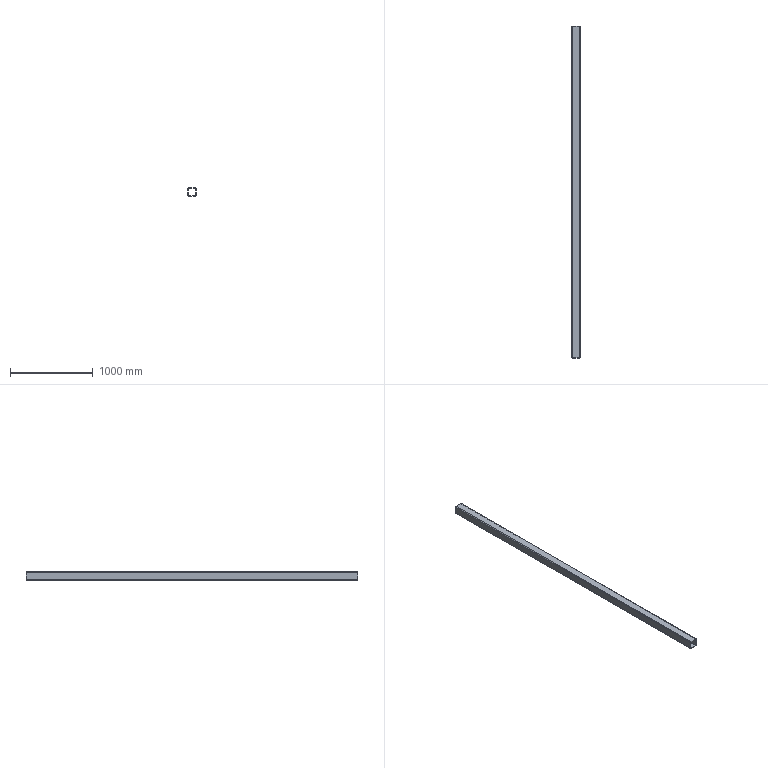Part | SolidWorks | features Extrusion 1 | 1 solid | 18 faces | box 100 x 4000 x 100 mm | volume 9368302 mm3 | plane 10 | cylinder 8 | commonest cylinder face diameters 12.6 x4 15.75 x4
STEP:
#1=CARTESIAN_POINT('',(100.,2000.,-90.6));
#2=VERTEX_POINT('',#1);
#3=CARTESIAN_POINT('',(92.125,2000.,-98.475));
#4=VERTEX_POINT('',#3);
#5=CARTESIAN_POINT('',(92.125,2000.,-90.6));
#6=DIRECTION('',(0.,1.,0.));
#7=DIRECTION('',(0.,0.,1.));
#8=AXIS2_PLACEMENT_3D('',#5,#6,#7);
#9=CIRCLE('',#8,7.875);
#10=EDGE_CURVE('',#2,#4,#9,.T.);
#11=ORIENTED_EDGE('',*,*,#10,.T.);
#12=CARTESIAN_POINT('',(7.875,2000.,-98.475));
#13=VERTEX_POINT('',#12);
#14=CARTESIAN_POINT('',(92.125,2000.,-98.475));
#15=DIRECTION('',(-1.,0.,0.));
#16=VECTOR('',#15,1000.);
#17=LINE('',#14,#16);
#18=EDGE_CURVE('',#4,#13,#17,.T.);
#19=ORIENTED_EDGE('',*,*,#18,.T.);
#20=CARTESIAN_POINT('',(0.,2000.,-90.6));
#21=VERTEX_POINT('',#20);
#22=CARTESIAN_POINT('',(7.875,2000.,-90.6));
#23=DIRECTION('',(0.,1.,0.));
#24=DIRECTION('',(0.,0.,1.));
#25=AXIS2_PLACEMENT_3D('',#22,#23,#24);
#26=CIRCLE('',#25,7.875);
#27=EDGE_CURVE('',#13,#21,#26,.T.);
#28=ORIENTED_EDGE('',*,*,#27,.T.);
#29=CARTESIAN_POINT('',(0.,2000.,-6.35));
#30=VERTEX_POINT('',#29);
#31=CARTESIAN_POINT('',(0.,2000.,-6.35));
#32=DIRECTION('',(0.,0.,1.));
#33=VECTOR('',#32,1000.);
#34=LINE('',#31,#33);
#35=EDGE_CURVE('',#21,#30,#34,.T.);
#36=ORIENTED_EDGE('',*,*,#35,.T.);
#37=CARTESIAN_POINT('',(7.875,2000.,1.525));
#38=VERTEX_POINT('',#37);
#39=CARTESIAN_POINT('',(7.875,2000.,-6.35));
#40=DIRECTION('',(0.,1.,0.));
#41=DIRECTION('',(0.,0.,1.));
#42=AXIS2_PLACEMENT_3D('',#39,#40,#41);
#43=CIRCLE('',#42,7.875);
#44=EDGE_CURVE('',#30,#38,#43,.T.);
#45=ORIENTED_EDGE('',*,*,#44,.T.);
#46=CARTESIAN_POINT('',(92.125,2000.,1.525));
#47=VERTEX_POINT('',#46);
#48=CARTESIAN_POINT('',(7.875,2000.,1.525));
#49=DIRECTION('',(1.,0.,0.));
#50=VECTOR('',#49,1000.);
#51=LINE('',#48,#50);
#52=EDGE_CURVE('',#38,#47,#51,.T.);
#53=ORIENTED_EDGE('',*,*,#52,.T.);
#54=CARTESIAN_POINT('',(100.,2000.,-6.35));
#55=VERTEX_POINT('',#54);
#56=CARTESIAN_POINT('',(92.125,2000.,-6.35));
#57=DIRECTION('',(0.,1.,0.));
#58=DIRECTION('',(0.,0.,1.));
#59=AXIS2_PLACEMENT_3D('',#56,#57,#58);
#60=CIRCLE('',#59,7.875);
#61=EDGE_CURVE('',#47,#55,#60,.T.);
#62=ORIENTED_EDGE('',*,*,#61,.T.);
#63=CARTESIAN_POINT('',(100.,2000.,-90.6));
#64=DIRECTION('',(0.,0.,-1.));
#65=VECTOR('',#64,1000.);
#66=LINE('',#63,#65);
#67=EDGE_CURVE('',#55,#2,#66,.T.);
#68=ORIENTED_EDGE('',*,*,#67,.T.);
#69=EDGE_LOOP('',(#11,#19,#28,#36,#45,#53,#62,#68));
#70=FACE_OUTER_BOUND('',#69,.T.);
#71=CARTESIAN_POINT('',(6.3,2000.,-85.875));
#72=VERTEX_POINT('',#71);
#73=CARTESIAN_POINT('',(6.3,2000.,-11.075));
#74=VERTEX_POINT('',#73);
#75=CARTESIAN_POINT('',(6.3,2000.,-11.075));
#76=DIRECTION('',(0.,0.,1.));
#77=VECTOR('',#76,1000.);
#78=LINE('',#75,#77);
#79=EDGE_CURVE('',#72,#74,#78,.T.);
#80=ORIENTED_EDGE('',*,*,#79,.F.);
#81=CARTESIAN_POINT('',(12.6,2000.,-92.175));
#82=VERTEX_POINT('',#81);
#83=CARTESIAN_POINT('',(12.6,2000.,-85.875));
#84=DIRECTION('',(0.,1.,0.));
#85=DIRECTION('',(0.,0.,1.));
#86=AXIS2_PLACEMENT_3D('',#83,#84,#85);
#87=CIRCLE('',#86,6.3);
#88=EDGE_CURVE('',#82,#72,#87,.T.);
#89=ORIENTED_EDGE('',*,*,#88,.F.);
#90=CARTESIAN_POINT('',(87.4,2000.,-92.175));
#91=VERTEX_POINT('',#90);
#92=CARTESIAN_POINT('',(87.4,2000.,-92.175));
#93=DIRECTION('',(-1.,0.,0.));
#94=VECTOR('',#93,1000.);
#95=LINE('',#92,#94);
#96=EDGE_CURVE('',#91,#82,#95,.T.);
#97=ORIENTED_EDGE('',*,*,#96,.F.);
#98=CARTESIAN_POINT('',(93.7,2000.,-85.875));
#99=VERTEX_POINT('',#98);
#100=CARTESIAN_POINT('',(87.4,2000.,-85.875));
#101=DIRECTION('',(0.,1.,0.));
#102=DIRECTION('',(0.,0.,1.));
#103=AXIS2_PLACEMENT_3D('',#100,#101,#102);
#104=CIRCLE('',#103,6.3);
#105=EDGE_CURVE('',#99,#91,#104,.T.);
#106=ORIENTED_EDGE('',*,*,#105,.F.);
#107=CARTESIAN_POINT('',(93.7,2000.,-11.075));
#108=VERTEX_POINT('',#107);
#109=CARTESIAN_POINT('',(93.7,2000.,-85.875));
#110=DIRECTION('',(0.,0.,-1.));
#111=VECTOR('',#110,1000.);
#112=LINE('',#109,#111);
#113=EDGE_CURVE('',#108,#99,#112,.T.);
#114=ORIENTED_EDGE('',*,*,#113,.F.);
#115=CARTESIAN_POINT('',(87.4,2000.,-4.775));
#116=VERTEX_POINT('',#115);
#117=CARTESIAN_POINT('',(87.4,2000.,-11.075));
#118=DIRECTION('',(0.,1.,0.));
#119=DIRECTION('',(0.,0.,1.));
#120=AXIS2_PLACEMENT_3D('',#117,#118,#119);
#121=CIRCLE('',#120,6.3);
#122=EDGE_CURVE('',#116,#108,#121,.T.);
#123=ORIENTED_EDGE('',*,*,#122,.F.);
#124=CARTESIAN_POINT('',(12.6,2000.,-4.775));
#125=VERTEX_POINT('',#124);
#126=CARTESIAN_POINT('',(12.6,2000.,-4.775));
#127=DIRECTION('',(1.,0.,0.));
#128=VECTOR('',#127,1000.);
#129=LINE('',#126,#128);
#130=EDGE_CURVE('',#125,#116,#129,.T.);
#131=ORIENTED_EDGE('',*,*,#130,.F.);
#132=CARTESIAN_POINT('',(12.6,2000.,-11.075));
#133=DIRECTION('',(0.,1.,0.));
#134=DIRECTION('',(0.,0.,1.));
#135=AXIS2_PLACEMENT_3D('',#132,#133,#134);
#136=CIRCLE('',#135,6.3);
#137=EDGE_CURVE('',#74,#125,#136,.T.);
#138=ORIENTED_EDGE('',*,*,#137,.F.);
#139=EDGE_LOOP('',(#80,#89,#97,#106,#114,#123,#131,#138));
#140=FACE_BOUND('',#139,.T.);
#141=CARTESIAN_POINT('',(92.125,2000.,-90.6));
#142=DIRECTION('',(0.,1.,0.));
#143=DIRECTION('',(0.,0.,1.));
#144=AXIS2_PLACEMENT_3D('',#141,#142,#143);
#145=PLANE('',#144);
#146=ADVANCED_FACE('',(#70,#140),#145,.T.);
#147=CARTESIAN_POINT('',(100.,-2000.,-90.6));
#148=VERTEX_POINT('',#147);
#149=CARTESIAN_POINT('',(92.125,-2000.,-98.475));
#150=VERTEX_POINT('',#149);
#151=CARTESIAN_POINT('',(92.125,-2000.,-90.6));
#152=DIRECTION('',(0.,1.,0.));
#153=DIRECTION('',(0.,0.,1.));
#154=AXIS2_PLACEMENT_3D('',#151,#152,#153);
#155=CIRCLE('',#154,7.875);
#156=EDGE_CURVE('',#148,#150,#155,.T.);
#157=ORIENTED_EDGE('',*,*,#156,.F.);
#158=CARTESIAN_POINT('',(100.,-2000.,-6.35));
#159=VERTEX_POINT('',#158);
#160=CARTESIAN_POINT('',(100.,-2000.,-90.6));
#161=DIRECTION('',(0.,0.,-1.));
#162=VECTOR('',#161,1000.);
#163=LINE('',#160,#162);
#164=EDGE_CURVE('',#159,#148,#163,.T.);
#165=ORIENTED_EDGE('',*,*,#164,.F.);
#166=CARTESIAN_POINT('',(92.125,-2000.,1.525));
#167=VERTEX_POINT('',#166);
#168=CARTESIAN_POINT('',(92.125,-2000.,-6.35));
#169=DIRECTION('',(0.,1.,0.));
#170=DIRECTION('',(0.,0.,1.));
#171=AXIS2_PLACEMENT_3D('',#168,#169,#170);
#172=CIRCLE('',#171,7.875);
#173=EDGE_CURVE('',#167,#159,#172,.T.);
#174=ORIENTED_EDGE('',*,*,#173,.F.);
#175=CARTESIAN_POINT('',(7.875,-2000.,1.525));
#176=VERTEX_POINT('',#175);
#177=CARTESIAN_POINT('',(7.875,-2000.,1.525));
#178=DIRECTION('',(1.,0.,0.));
#179=VECTOR('',#178,1000.);
#180=LINE('',#177,#179);
#181=EDGE_CURVE('',#176,#167,#180,.T.);
#182=ORIENTED_EDGE('',*,*,#181,.F.);
#183=CARTESIAN_POINT('',(0.,-2000.,-6.35));
#184=VERTEX_POINT('',#183);
#185=CARTESIAN_POINT('',(7.875,-2000.,-6.35));
#186=DIRECTION('',(0.,1.,0.));
#187=DIRECTION('',(0.,0.,1.));
#188=AXIS2_PLACEMENT_3D('',#185,#186,#187);
#189=CIRCLE('',#188,7.875);
#190=EDGE_CURVE('',#184,#176,#189,.T.);
#191=ORIENTED_EDGE('',*,*,#190,.F.);
#192=CARTESIAN_POINT('',(0.,-2000.,-90.6));
#193=VERTEX_POINT('',#192);
#194=CARTESIAN_POINT('',(0.,-2000.,-6.35));
#195=DIRECTION('',(0.,0.,1.));
#196=VECTOR('',#195,1000.);
#197=LINE('',#194,#196);
#198=EDGE_CURVE('',#193,#184,#197,.T.);
#199=ORIENTED_EDGE('',*,*,#198,.F.);
#200=CARTESIAN_POINT('',(7.875,-2000.,-98.475));
#201=VERTEX_POINT('',#200);
#202=CARTESIAN_POINT('',(7.875,-2000.,-90.6));
#203=DIRECTION('',(0.,1.,0.));
#204=DIRECTION('',(0.,0.,1.));
#205=AXIS2_PLACEMENT_3D('',#202,#203,#204);
#206=CIRCLE('',#205,7.875);
#207=EDGE_CURVE('',#201,#193,#206,.T.);
#208=ORIENTED_EDGE('',*,*,#207,.F.);
#209=CARTESIAN_POINT('',(92.125,-2000.,-98.475));
#210=DIRECTION('',(-1.,0.,0.));
#211=VECTOR('',#210,1000.);
#212=LINE('',#209,#211);
#213=EDGE_CURVE('',#150,#201,#212,.T.);
#214=ORIENTED_EDGE('',*,*,#213,.F.);
#215=EDGE_LOOP('',(#157,#165,#174,#182,#191,#199,#208,#214));
#216=FACE_OUTER_BOUND('',#215,.T.);
#217=CARTESIAN_POINT('',(12.6,-2000.,-92.175));
#218=VERTEX_POINT('',#217);
#219=CARTESIAN_POINT('',(6.3,-2000.,-85.875));
#220=VERTEX_POINT('',#219);
#221=CARTESIAN_POINT('',(12.6,-2000.,-85.875));
#222=DIRECTION('',(0.,1.,0.));
#223=DIRECTION('',(0.,0.,1.));
#224=AXIS2_PLACEMENT_3D('',#221,#222,#223);
#225=CIRCLE('',#224,6.3);
#226=EDGE_CURVE('',#218,#220,#225,.T.);
#227=ORIENTED_EDGE('',*,*,#226,.T.);
#228=CARTESIAN_POINT('',(6.3,-2000.,-11.075));
#229=VERTEX_POINT('',#228);
#230=CARTESIAN_POINT('',(6.3,-2000.,-11.075));
#231=DIRECTION('',(0.,0.,1.));
#232=VECTOR('',#231,1000.);
#233=LINE('',#230,#232);
#234=EDGE_CURVE('',#220,#229,#233,.T.);
#235=ORIENTED_EDGE('',*,*,#234,.T.);
#236=CARTESIAN_POINT('',(12.6,-2000.,-4.775));
#237=VERTEX_POINT('',#236);
#238=CARTESIAN_POINT('',(12.6,-2000.,-11.075));
#239=DIRECTION('',(0.,1.,0.));
#240=DIRECTION('',(0.,0.,1.));
#241=AXIS2_PLACEMENT_3D('',#238,#239,#240);
#242=CIRCLE('',#241,6.3);
#243=EDGE_CURVE('',#229,#237,#242,.T.);
#244=ORIENTED_EDGE('',*,*,#243,.T.);
#245=CARTESIAN_POINT('',(87.4,-2000.,-4.775));
#246=VERTEX_POINT('',#245);
#247=CARTESIAN_POINT('',(12.6,-2000.,-4.775));
#248=DIRECTION('',(1.,0.,0.));
#249=VECTOR('',#248,1000.);
#250=LINE('',#247,#249);
#251=EDGE_CURVE('',#237,#246,#250,.T.);
#252=ORIENTED_EDGE('',*,*,#251,.T.);
#253=CARTESIAN_POINT('',(93.7,-2000.,-11.075));
#254=VERTEX_POINT('',#253);
#255=CARTESIAN_POINT('',(87.4,-2000.,-11.075));
#256=DIRECTION('',(0.,1.,0.));
#257=DIRECTION('',(0.,0.,1.));
#258=AXIS2_PLACEMENT_3D('',#255,#256,#257);
#259=CIRCLE('',#258,6.3);
#260=EDGE_CURVE('',#246,#254,#259,.T.);
#261=ORIENTED_EDGE('',*,*,#260,.T.);
#262=CARTESIAN_POINT('',(93.7,-2000.,-85.875));
#263=VERTEX_POINT('',#262);
#264=CARTESIAN_POINT('',(93.7,-2000.,-85.875));
#265=DIRECTION('',(0.,0.,-1.));
#266=VECTOR('',#265,1000.);
#267=LINE('',#264,#266);
#268=EDGE_CURVE('',#254,#263,#267,.T.);
#269=ORIENTED_EDGE('',*,*,#268,.T.);
#270=CARTESIAN_POINT('',(87.4,-2000.,-92.175));
#271=VERTEX_POINT('',#270);
#272=CARTESIAN_POINT('',(87.4,-2000.,-85.875));
#273=DIRECTION('',(0.,1.,0.));
#274=DIRECTION('',(0.,0.,1.));
#275=AXIS2_PLACEMENT_3D('',#272,#273,#274);
#276=CIRCLE('',#275,6.3);
#277=EDGE_CURVE('',#263,#271,#276,.T.);
#278=ORIENTED_EDGE('',*,*,#277,.T.);
#279=CARTESIAN_POINT('',(87.4,-2000.,-92.175));
#280=DIRECTION('',(-1.,0.,0.));
#281=VECTOR('',#280,1000.);
#282=LINE('',#279,#281);
#283=EDGE_CURVE('',#271,#218,#282,.T.);
#284=ORIENTED_EDGE('',*,*,#283,.T.);
#285=EDGE_LOOP('',(#227,#235,#244,#252,#261,#269,#278,#284));
#286=FACE_BOUND('',#285,.T.);
#287=CARTESIAN_POINT('',(92.125,-2000.,-90.6));
#288=DIRECTION('',(0.,1.,0.));
#289=DIRECTION('',(0.,0.,1.));
#290=AXIS2_PLACEMENT_3D('',#287,#288,#289);
#291=PLANE('',#290);
#292=ADVANCED_FACE('',(#216,#286),#291,.F.);
#293=ORIENTED_EDGE('',*,*,#156,.T.);
#294=CARTESIAN_POINT('',(92.125,2000.,-98.475));
#295=DIRECTION('',(0.,-1.,0.));
#296=VECTOR('',#295,1000.);
#297=LINE('',#294,#296);
#298=EDGE_CURVE('',#4,#150,#297,.T.);
#299=ORIENTED_EDGE('',*,*,#298,.F.);
#300=ORIENTED_EDGE('',*,*,#10,.F.);
#301=CARTESIAN_POINT('',(100.,2000.,-90.6));
#302=DIRECTION('',(0.,-1.,0.));
#303=VECTOR('',#302,1000.);
#304=LINE('',#301,#303);
#305=EDGE_CURVE('',#2,#148,#304,.T.);
#306=ORIENTED_EDGE('',*,*,#305,.T.);
#307=EDGE_LOOP('',(#293,#299,#300,#306));
#308=FACE_OUTER_BOUND('',#307,.T.);
#309=CARTESIAN_POINT('',(92.125,2000.,-90.6));
#310=DIRECTION('',(0.,-1.,0.));
#311=DIRECTION('',(0.,0.,-1.));
#312=AXIS2_PLACEMENT_3D('',#309,#310,#311);
#313=CYLINDRICAL_SURFACE('',#312,7.875);
#314=ADVANCED_FACE('',(#308),#313,.T.);
#315=ORIENTED_EDGE('',*,*,#213,.T.);
#316=CARTESIAN_POINT('',(7.875,2000.,-98.475));
#317=DIRECTION('',(0.,-1.,0.));
#318=VECTOR('',#317,1000.);
#319=LINE('',#316,#318);
#320=EDGE_CURVE('',#13,#201,#319,.T.);
#321=ORIENTED_EDGE('',*,*,#320,.F.);
#322=ORIENTED_EDGE('',*,*,#18,.F.);
#323=ORIENTED_EDGE('',*,*,#298,.T.);
#324=EDGE_LOOP('',(#315,#321,#322,#323));
#325=FACE_OUTER_BOUND('',#324,.T.);
#326=CARTESIAN_POINT('',(92.125,2000.,-98.475));
#327=DIRECTION('',(0.,0.,1.));
#328=DIRECTION('',(1.,0.,0.));
#329=AXIS2_PLACEMENT_3D('',#326,#327,#328);
#330=PLANE('',#329);
#331=ADVANCED_FACE('',(#325),#330,.F.);
#332=ORIENTED_EDGE('',*,*,#207,.T.);
#333=CARTESIAN_POINT('',(0.,2000.,-90.6));
#334=DIRECTION('',(0.,-1.,0.));
#335=VECTOR('',#334,1000.);
#336=LINE('',#333,#335);
#337=EDGE_CURVE('',#21,#193,#336,.T.);
#338=ORIENTED_EDGE('',*,*,#337,.F.);
#339=ORIENTED_EDGE('',*,*,#27,.F.);
#340=ORIENTED_EDGE('',*,*,#320,.T.);
#341=EDGE_LOOP('',(#332,#338,#339,#340));
#342=FACE_OUTER_BOUND('',#341,.T.);
#343=CARTESIAN_POINT('',(7.875,2000.,-90.6));
#344=DIRECTION('',(0.,-1.,0.));
#345=DIRECTION('',(0.,0.,-1.));
#346=AXIS2_PLACEMENT_3D('',#343,#344,#345);
#347=CYLINDRICAL_SURFACE('',#346,7.875);
#348=ADVANCED_FACE('',(#342),#347,.T.);
#349=ORIENTED_EDGE('',*,*,#198,.T.);
#350=CARTESIAN_POINT('',(0.,2000.,-6.35));
#351=DIRECTION('',(0.,-1.,0.));
#352=VECTOR('',#351,1000.);
#353=LINE('',#350,#352);
#354=EDGE_CURVE('',#30,#184,#353,.T.);
#355=ORIENTED_EDGE('',*,*,#354,.F.);
#356=ORIENTED_EDGE('',*,*,#35,.F.);
#357=ORIENTED_EDGE('',*,*,#337,.T.);
#358=EDGE_LOOP('',(#349,#355,#356,#357));
#359=FACE_OUTER_BOUND('',#358,.T.);
#360=CARTESIAN_POINT('',(0.,2000.,-6.35));
#361=DIRECTION('',(1.,0.,0.));
#362=DIRECTION('',(0.,0.,-1.));
#363=AXIS2_PLACEMENT_3D('',#360,#361,#362);
#364=PLANE('',#363);
#365=ADVANCED_FACE('',(#359),#364,.F.);
#366=ORIENTED_EDGE('',*,*,#190,.T.);
#367=CARTESIAN_POINT('',(7.875,2000.,1.525));
#368=DIRECTION('',(0.,-1.,0.));
#369=VECTOR('',#368,1000.);
#370=LINE('',#367,#369);
#371=EDGE_CURVE('',#38,#176,#370,.T.);
#372=ORIENTED_EDGE('',*,*,#371,.F.);
#373=ORIENTED_EDGE('',*,*,#44,.F.);
#374=ORIENTED_EDGE('',*,*,#354,.T.);
#375=EDGE_LOOP('',(#366,#372,#373,#374));
#376=FACE_OUTER_BOUND('',#375,.T.);
#377=CARTESIAN_POINT('',(7.875,2000.,-6.35));
#378=DIRECTION('',(0.,-1.,0.));
#379=DIRECTION('',(0.,0.,-1.));
#380=AXIS2_PLACEMENT_3D('',#377,#378,#379);
#381=CYLINDRICAL_SURFACE('',#380,7.875);
#382=ADVANCED_FACE('',(#376),#381,.T.);
#383=ORIENTED_EDGE('',*,*,#181,.T.);
#384=CARTESIAN_POINT('',(92.125,2000.,1.525));
#385=DIRECTION('',(0.,-1.,0.));
#386=VECTOR('',#385,1000.);
#387=LINE('',#384,#386);
#388=EDGE_CURVE('',#47,#167,#387,.T.);
#389=ORIENTED_EDGE('',*,*,#388,.F.);
#390=ORIENTED_EDGE('',*,*,#52,.F.);
#391=ORIENTED_EDGE('',*,*,#371,.T.);
#392=EDGE_LOOP('',(#383,#389,#390,#391));
#393=FACE_OUTER_BOUND('',#392,.T.);
#394=CARTESIAN_POINT('',(7.875,2000.,1.525));
#395=DIRECTION('',(0.,0.,-1.));
#396=DIRECTION('',(-1.,0.,0.));
#397=AXIS2_PLACEMENT_3D('',#394,#395,#396);
#398=PLANE('',#397);
#399=ADVANCED_FACE('',(#393),#398,.F.);
#400=ORIENTED_EDGE('',*,*,#173,.T.);
#401=CARTESIAN_POINT('',(100.,2000.,-6.35));
#402=DIRECTION('',(0.,-1.,0.));
#403=VECTOR('',#402,1000.);
#404=LINE('',#401,#403);
#405=EDGE_CURVE('',#55,#159,#404,.T.);
#406=ORIENTED_EDGE('',*,*,#405,.F.);
#407=ORIENTED_EDGE('',*,*,#61,.F.);
#408=ORIENTED_EDGE('',*,*,#388,.T.);
#409=EDGE_LOOP('',(#400,#406,#407,#408));
#410=FACE_OUTER_BOUND('',#409,.T.);
#411=CARTESIAN_POINT('',(92.125,2000.,-6.35));
#412=DIRECTION('',(0.,-1.,0.));
#413=DIRECTION('',(0.,0.,-1.));
#414=AXIS2_PLACEMENT_3D('',#411,#412,#413);
#415=CYLINDRICAL_SURFACE('',#414,7.875);
#416=ADVANCED_FACE('',(#410),#415,.T.);
#417=ORIENTED_EDGE('',*,*,#164,.T.);
#418=ORIENTED_EDGE('',*,*,#305,.F.);
#419=ORIENTED_EDGE('',*,*,#67,.F.);
#420=ORIENTED_EDGE('',*,*,#405,.T.);
#421=EDGE_LOOP('',(#417,#418,#419,#420));
#422=FACE_OUTER_BOUND('',#421,.T.);
#423=CARTESIAN_POINT('',(100.,2000.,-90.6));
#424=DIRECTION('',(-1.,0.,0.));
#425=DIRECTION('',(0.,0.,1.));
#426=AXIS2_PLACEMENT_3D('',#423,#424,#425);
#427=PLANE('',#426);
#428=ADVANCED_FACE('',(#422),#427,.F.);
#429=ORIENTED_EDGE('',*,*,#226,.F.);
#430=CARTESIAN_POINT('',(12.6,2000.,-92.175));
#431=DIRECTION('',(0.,-1.,0.));
#432=VECTOR('',#431,1000.);
#433=LINE('',#430,#432);
#434=EDGE_CURVE('',#82,#218,#433,.T.);
#435=ORIENTED_EDGE('',*,*,#434,.F.);
#436=ORIENTED_EDGE('',*,*,#88,.T.);
#437=CARTESIAN_POINT('',(6.3,2000.,-85.875));
#438=DIRECTION('',(0.,-1.,0.));
#439=VECTOR('',#438,1000.);
#440=LINE('',#437,#439);
#441=EDGE_CURVE('',#72,#220,#440,.T.);
#442=ORIENTED_EDGE('',*,*,#441,.T.);
#443=EDGE_LOOP('',(#429,#435,#436,#442));
#444=FACE_OUTER_BOUND('',#443,.T.);
#445=CARTESIAN_POINT('',(12.6,2000.,-85.875));
#446=DIRECTION('',(0.,-1.,0.));
#447=DIRECTION('',(0.,0.,-1.));
#448=AXIS2_PLACEMENT_3D('',#445,#446,#447);
#449=CYLINDRICAL_SURFACE('',#448,6.3);
#450=ADVANCED_FACE('',(#444),#449,.F.);
#451=ORIENTED_EDGE('',*,*,#234,.F.);
#452=ORIENTED_EDGE('',*,*,#441,.F.);
#453=ORIENTED_EDGE('',*,*,#79,.T.);
#454=CARTESIAN_POINT('',(6.3,2000.,-11.075));
#455=DIRECTION('',(0.,-1.,0.));
#456=VECTOR('',#455,1000.);
#457=LINE('',#454,#456);
#458=EDGE_CURVE('',#74,#229,#457,.T.);
#459=ORIENTED_EDGE('',*,*,#458,.T.);
#460=EDGE_LOOP('',(#451,#452,#453,#459));
#461=FACE_OUTER_BOUND('',#460,.T.);
#462=CARTESIAN_POINT('',(6.3,2000.,-11.075));
#463=DIRECTION('',(1.,0.,0.));
#464=DIRECTION('',(0.,0.,-1.));
#465=AXIS2_PLACEMENT_3D('',#462,#463,#464);
#466=PLANE('',#465);
#467=ADVANCED_FACE('',(#461),#466,.T.);
#468=ORIENTED_EDGE('',*,*,#243,.F.);
#469=ORIENTED_EDGE('',*,*,#458,.F.);
#470=ORIENTED_EDGE('',*,*,#137,.T.);
#471=CARTESIAN_POINT('',(12.6,2000.,-4.775));
#472=DIRECTION('',(0.,-1.,0.));
#473=VECTOR('',#472,1000.);
#474=LINE('',#471,#473);
#475=EDGE_CURVE('',#125,#237,#474,.T.);
#476=ORIENTED_EDGE('',*,*,#475,.T.);
#477=EDGE_LOOP('',(#468,#469,#470,#476));
#478=FACE_OUTER_BOUND('',#477,.T.);
#479=CARTESIAN_POINT('',(12.6,2000.,-11.075));
#480=DIRECTION('',(0.,-1.,0.));
#481=DIRECTION('',(0.,0.,-1.));
#482=AXIS2_PLACEMENT_3D('',#479,#480,#481);
#483=CYLINDRICAL_SURFACE('',#482,6.3);
#484=ADVANCED_FACE('',(#478),#483,.F.);
#485=ORIENTED_EDGE('',*,*,#251,.F.);
#486=ORIENTED_EDGE('',*,*,#475,.F.);
#487=ORIENTED_EDGE('',*,*,#130,.T.);
#488=CARTESIAN_POINT('',(87.4,2000.,-4.775));
#489=DIRECTION('',(0.,-1.,0.));
#490=VECTOR('',#489,1000.);
#491=LINE('',#488,#490);
#492=EDGE_CURVE('',#116,#246,#491,.T.);
#493=ORIENTED_EDGE('',*,*,#492,.T.);
#494=EDGE_LOOP('',(#485,#486,#487,#493));
#495=FACE_OUTER_BOUND('',#494,.T.);
#496=CARTESIAN_POINT('',(12.6,2000.,-4.775));
#497=DIRECTION('',(0.,0.,-1.));
#498=DIRECTION('',(-1.,0.,0.));
#499=AXIS2_PLACEMENT_3D('',#496,#497,#498);
#500=PLANE('',#499);
#501=ADVANCED_FACE('',(#495),#500,.T.);
#502=ORIENTED_EDGE('',*,*,#260,.F.);
#503=ORIENTED_EDGE('',*,*,#492,.F.);
#504=ORIENTED_EDGE('',*,*,#122,.T.);
#505=CARTESIAN_POINT('',(93.7,2000.,-11.075));
#506=DIRECTION('',(0.,-1.,0.));
#507=VECTOR('',#506,1000.);
#508=LINE('',#505,#507);
#509=EDGE_CURVE('',#108,#254,#508,.T.);
#510=ORIENTED_EDGE('',*,*,#509,.T.);
#511=EDGE_LOOP('',(#502,#503,#504,#510));
#512=FACE_OUTER_BOUND('',#511,.T.);
#513=CARTESIAN_POINT('',(87.4,2000.,-11.075));
#514=DIRECTION('',(0.,-1.,0.));
#515=DIRECTION('',(0.,0.,-1.));
#516=AXIS2_PLACEMENT_3D('',#513,#514,#515);
#517=CYLINDRICAL_SURFACE('',#516,6.3);
#518=ADVANCED_FACE('',(#512),#517,.F.);
#519=ORIENTED_EDGE('',*,*,#268,.F.);
#520=ORIENTED_EDGE('',*,*,#509,.F.);
#521=ORIENTED_EDGE('',*,*,#113,.T.);
#522=CARTESIAN_POINT('',(93.7,2000.,-85.875));
#523=DIRECTION('',(0.,-1.,0.));
#524=VECTOR('',#523,1000.);
#525=LINE('',#522,#524);
#526=EDGE_CURVE('',#99,#263,#525,.T.);
#527=ORIENTED_EDGE('',*,*,#526,.T.);
#528=EDGE_LOOP('',(#519,#520,#521,#527));
#529=FACE_OUTER_BOUND('',#528,.T.);
#530=CARTESIAN_POINT('',(93.7,2000.,-85.875));
#531=DIRECTION('',(-1.,0.,0.));
#532=DIRECTION('',(0.,0.,1.));
#533=AXIS2_PLACEMENT_3D('',#530,#531,#532);
#534=PLANE('',#533);
#535=ADVANCED_FACE('',(#529),#534,.T.);
#536=ORIENTED_EDGE('',*,*,#277,.F.);
#537=ORIENTED_EDGE('',*,*,#526,.F.);
#538=ORIENTED_EDGE('',*,*,#105,.T.);
#539=CARTESIAN_POINT('',(87.4,2000.,-92.175));
#540=DIRECTION('',(0.,-1.,0.));
#541=VECTOR('',#540,1000.);
#542=LINE('',#539,#541);
#543=EDGE_CURVE('',#91,#271,#542,.T.);
#544=ORIENTED_EDGE('',*,*,#543,.T.);
#545=EDGE_LOOP('',(#536,#537,#538,#544));
#546=FACE_OUTER_BOUND('',#545,.T.);
#547=CARTESIAN_POINT('',(87.4,2000.,-85.875));
#548=DIRECTION('',(0.,-1.,0.));
#549=DIRECTION('',(0.,0.,-1.));
#550=AXIS2_PLACEMENT_3D('',#547,#548,#549);
#551=CYLINDRICAL_SURFACE('',#550,6.3);
#552=ADVANCED_FACE('',(#546),#551,.F.);
#553=ORIENTED_EDGE('',*,*,#283,.F.);
#554=ORIENTED_EDGE('',*,*,#543,.F.);
#555=ORIENTED_EDGE('',*,*,#96,.T.);
#556=ORIENTED_EDGE('',*,*,#434,.T.);
#557=EDGE_LOOP('',(#553,#554,#555,#556));
#558=FACE_OUTER_BOUND('',#557,.T.);
#559=CARTESIAN_POINT('',(87.4,2000.,-92.175));
#560=DIRECTION('',(0.,0.,1.));
#561=DIRECTION('',(1.,0.,0.));
#562=AXIS2_PLACEMENT_3D('',#559,#560,#561);
#563=PLANE('',#562);
#564=ADVANCED_FACE('',(#558),#563,.T.);
#565=CLOSED_SHELL('',(#146,#292,#314,#331,#348,#365,#382,#399,#416,#428,#450,#467,#484,#501,#518,#535,#552,#564));
#566=MANIFOLD_SOLID_BREP('',#565);
#567=CARTESIAN_POINT('',(0.,0.,0.));
#568=DIRECTION('',(0.,0.,1.));
#569=DIRECTION('',(1.,0.,0.));
#570=AXIS2_PLACEMENT_3D('',#567,#568,#569);
#571=(LENGTH_UNIT()NAMED_UNIT(*)SI_UNIT(.MILLI.,.METRE.));
#572=UNCERTAINTY_MEASURE_WITH_UNIT(LENGTH_MEASURE(0.00001),#571,'','');
#573=(NAMED_UNIT(*)PLANE_ANGLE_UNIT()SI_UNIT($,.RADIAN.));
#574=(NAMED_UNIT(*)SI_UNIT($,.STERADIAN.)SOLID_ANGLE_UNIT());
#575=(GEOMETRIC_REPRESENTATION_CONTEXT(3)GLOBAL_UNCERTAINTY_ASSIGNED_CONTEXT((#572))GLOBAL_UNIT_ASSIGNED_CONTEXT((#571,#573,#574))REPRESENTATION_CONTEXT('',''));
#576=ADVANCED_BREP_SHAPE_REPRESENTATION('',(#566,#570),#575);